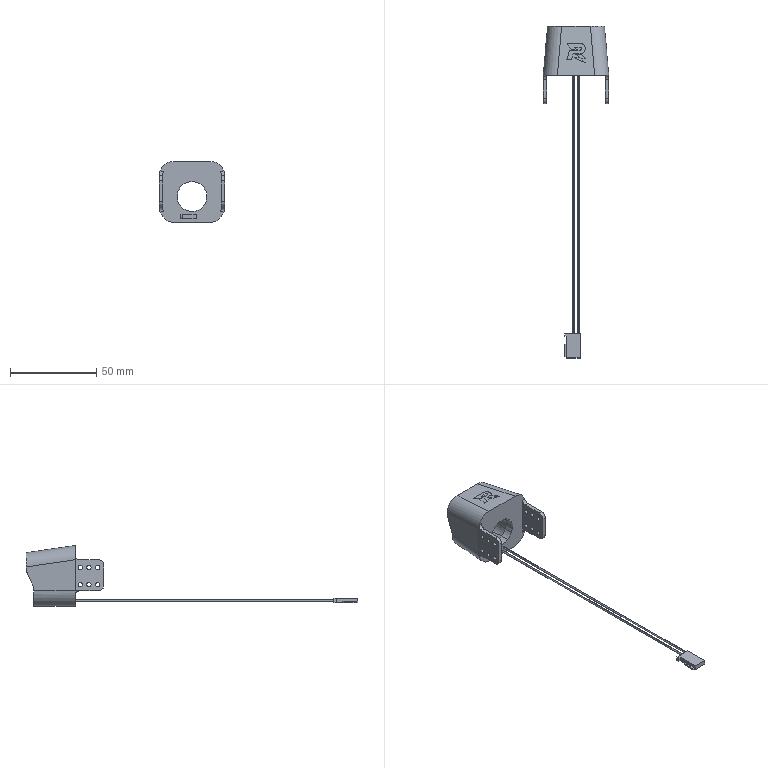Part | SolidWorks | features BaseBody 1 | 1 solid | 158 faces | box 37.988 x 192.5 x 35.318 mm | volume 21359 mm3 | plane 84 | cylinder 46 | spline 24 | cone 4 | commonest cylinder face diameters 2.5 x24 1 x4 5 x4 6 x4 12.44 x2 16.44 x2